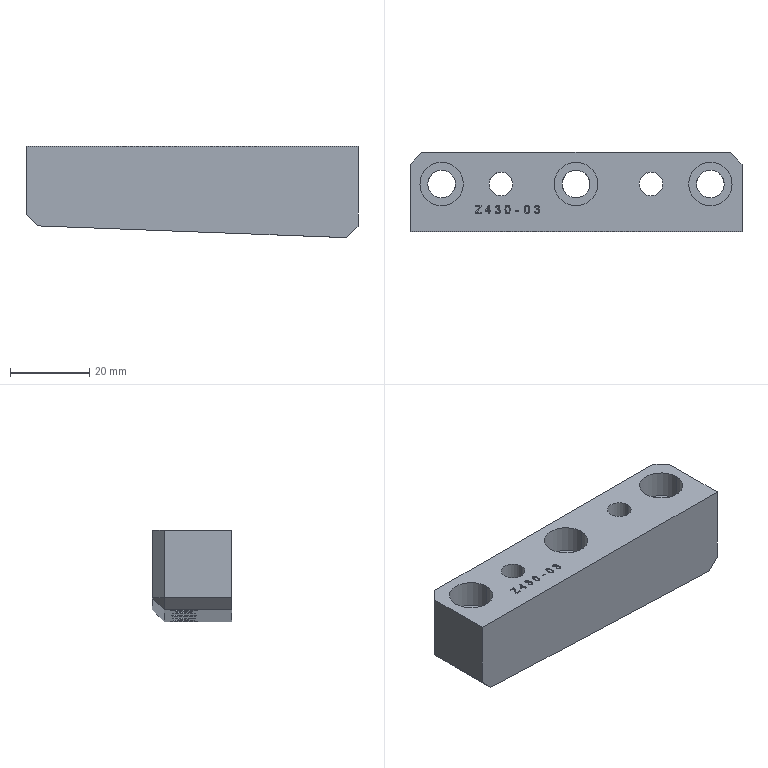Part | Creo | 1 solid | 172 faces | box 84 x 20 x 23.085 mm | volume 30662 mm3 | other 105 | plane 50 | cylinder 17 | commonest cylinder face diameters 7 x6 11 x6 6 x4 30.388 x1